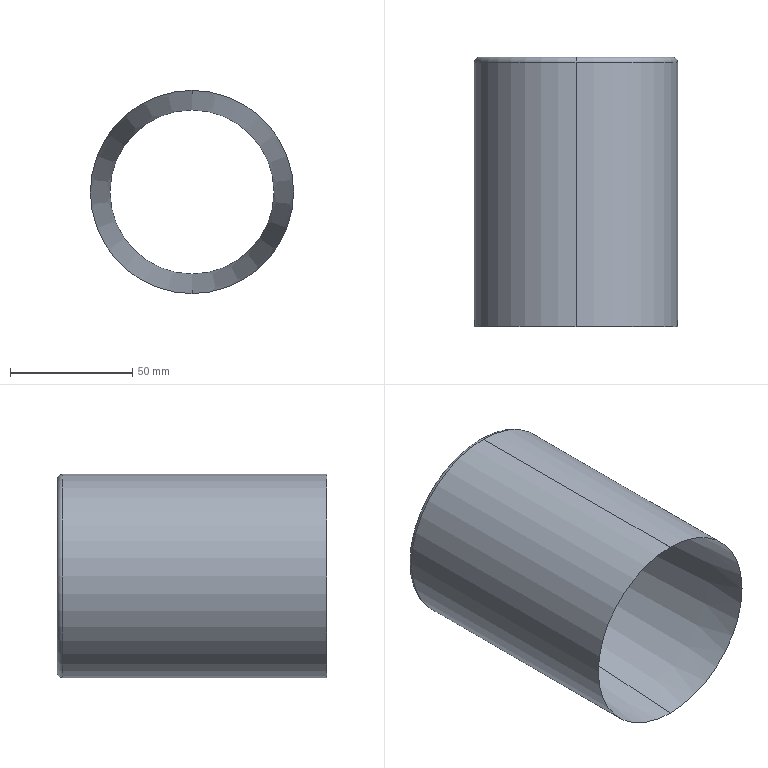Part | SolidWorks | features RevolutionThin 1 | 1 solid | 22 faces | box 83 x 110 x 83 mm | volume 48850 mm3 | cylinder 8 | torus 8 | cone 4 | plane 2 | commonest cylinder face diameters 67 x2 69 x2 81 x2 83 x2
STEP:
#1=CARTESIAN_POINT('',(0.,108.,33.5));
#2=VERTEX_POINT('',#1);
#3=CARTESIAN_POINT('',(0.,108.,-33.5));
#4=VERTEX_POINT('',#3);
#5=CARTESIAN_POINT('',(0.,108.,0.));
#6=DIRECTION('',(0.,-1.,0.));
#7=DIRECTION('',(0.,0.,-1.));
#8=AXIS2_PLACEMENT_3D('',#5,#6,#7);
#9=CIRCLE('',#8,33.5);
#10=EDGE_CURVE('',#2,#4,#9,.T.);
#11=ORIENTED_EDGE('',*,*,#10,.F.);
#12=CARTESIAN_POINT('',(0.,105.,33.5));
#13=VERTEX_POINT('',#12);
#14=CARTESIAN_POINT('',(0.,0.,33.5));
#15=DIRECTION('',(0.,-1.,0.));
#16=VECTOR('',#15,1000.);
#17=LINE('',#14,#16);
#18=EDGE_CURVE('',#2,#13,#17,.T.);
#19=ORIENTED_EDGE('',*,*,#18,.T.);
#20=CARTESIAN_POINT('',(0.,105.,-33.5));
#21=VERTEX_POINT('',#20);
#22=CARTESIAN_POINT('',(0.,105.,0.));
#23=DIRECTION('',(0.,-1.,0.));
#24=DIRECTION('',(0.,0.,-1.));
#25=AXIS2_PLACEMENT_3D('',#22,#23,#24);
#26=CIRCLE('',#25,33.5);
#27=EDGE_CURVE('',#13,#21,#26,.T.);
#28=ORIENTED_EDGE('',*,*,#27,.T.);
#29=CARTESIAN_POINT('',(0.,0.,-33.5));
#30=DIRECTION('',(0.,-1.,0.));
#31=VECTOR('',#30,1000.);
#32=LINE('',#29,#31);
#33=EDGE_CURVE('',#4,#21,#32,.T.);
#34=ORIENTED_EDGE('',*,*,#33,.F.);
#35=EDGE_LOOP('',(#11,#19,#28,#34));
#36=FACE_OUTER_BOUND('',#35,.T.);
#37=CARTESIAN_POINT('',(0.,0.,0.));
#38=DIRECTION('',(0.,-1.,0.));
#39=DIRECTION('',(0.,0.,-1.));
#40=AXIS2_PLACEMENT_3D('',#37,#38,#39);
#41=CYLINDRICAL_SURFACE('',#40,33.5);
#42=ADVANCED_FACE('',(#36),#41,.F.);
#43=CARTESIAN_POINT('',(0.,108.,0.));
#44=DIRECTION('',(0.,-1.,0.));
#45=DIRECTION('',(0.,0.,-1.));
#46=AXIS2_PLACEMENT_3D('',#43,#44,#45);
#47=CIRCLE('',#46,33.5);
#48=EDGE_CURVE('',#4,#2,#47,.T.);
#49=ORIENTED_EDGE('',*,*,#48,.T.);
#50=CARTESIAN_POINT('',(0.,110.,35.5));
#51=VERTEX_POINT('',#50);
#52=CARTESIAN_POINT('',(0.,108.,35.5));
#53=DIRECTION('',(1.,0.,0.));
#54=DIRECTION('',(0.,0.,-1.));
#55=AXIS2_PLACEMENT_3D('',#52,#53,#54);
#56=CIRCLE('',#55,2.);
#57=EDGE_CURVE('',#2,#51,#56,.T.);
#58=ORIENTED_EDGE('',*,*,#57,.T.);
#59=CARTESIAN_POINT('',(0.,110.,-35.5));
#60=VERTEX_POINT('',#59);
#61=CARTESIAN_POINT('',(0.,110.,0.));
#62=DIRECTION('',(0.,-1.,0.));
#63=DIRECTION('',(0.,0.,-1.));
#64=AXIS2_PLACEMENT_3D('',#61,#62,#63);
#65=CIRCLE('',#64,35.5);
#66=EDGE_CURVE('',#60,#51,#65,.T.);
#67=ORIENTED_EDGE('',*,*,#66,.F.);
#68=CARTESIAN_POINT('',(0.,108.,-35.5));
#69=DIRECTION('',(-1.,0.,0.));
#70=DIRECTION('',(0.,0.,1.));
#71=AXIS2_PLACEMENT_3D('',#68,#69,#70);
#72=CIRCLE('',#71,2.);
#73=EDGE_CURVE('',#4,#60,#72,.T.);
#74=ORIENTED_EDGE('',*,*,#73,.F.);
#75=EDGE_LOOP('',(#49,#58,#67,#74));
#76=FACE_OUTER_BOUND('',#75,.T.);
#77=CARTESIAN_POINT('',(0.,108.,0.));
#78=DIRECTION('',(0.,-1.,0.));
#79=DIRECTION('',(0.,0.,-1.));
#80=AXIS2_PLACEMENT_3D('',#77,#78,#79);
#81=TOROIDAL_SURFACE('',#80,35.5,2.);
#82=ADVANCED_FACE('',(#76),#81,.T.);
#83=CARTESIAN_POINT('',(0.,110.,-39.5));
#84=VERTEX_POINT('',#83);
#85=CARTESIAN_POINT('',(0.,110.,39.5));
#86=VERTEX_POINT('',#85);
#87=CARTESIAN_POINT('',(0.,110.,0.));
#88=DIRECTION('',(0.,-1.,0.));
#89=DIRECTION('',(0.,0.,-1.));
#90=AXIS2_PLACEMENT_3D('',#87,#88,#89);
#91=CIRCLE('',#90,39.5);
#92=EDGE_CURVE('',#84,#86,#91,.T.);
#93=ORIENTED_EDGE('',*,*,#92,.T.);
#94=CARTESIAN_POINT('',(0.,108.,41.5));
#95=VERTEX_POINT('',#94);
#96=CARTESIAN_POINT('',(0.,108.,39.5));
#97=DIRECTION('',(1.,0.,0.));
#98=DIRECTION('',(0.,0.,-1.));
#99=AXIS2_PLACEMENT_3D('',#96,#97,#98);
#100=CIRCLE('',#99,2.);
#101=EDGE_CURVE('',#86,#95,#100,.T.);
#102=ORIENTED_EDGE('',*,*,#101,.T.);
#103=CARTESIAN_POINT('',(0.,108.,-41.5));
#104=VERTEX_POINT('',#103);
#105=CARTESIAN_POINT('',(0.,108.,0.));
#106=DIRECTION('',(0.,-1.,0.));
#107=DIRECTION('',(0.,0.,-1.));
#108=AXIS2_PLACEMENT_3D('',#105,#106,#107);
#109=CIRCLE('',#108,41.5);
#110=EDGE_CURVE('',#104,#95,#109,.T.);
#111=ORIENTED_EDGE('',*,*,#110,.F.);
#112=CARTESIAN_POINT('',(0.,108.,-39.5));
#113=DIRECTION('',(-1.,0.,0.));
#114=DIRECTION('',(0.,0.,1.));
#115=AXIS2_PLACEMENT_3D('',#112,#113,#114);
#116=CIRCLE('',#115,2.);
#117=EDGE_CURVE('',#84,#104,#116,.T.);
#118=ORIENTED_EDGE('',*,*,#117,.F.);
#119=EDGE_LOOP('',(#93,#102,#111,#118));
#120=FACE_OUTER_BOUND('',#119,.T.);
#121=CARTESIAN_POINT('',(0.,108.,0.));
#122=DIRECTION('',(0.,-1.,0.));
#123=DIRECTION('',(0.,0.,-1.));
#124=AXIS2_PLACEMENT_3D('',#121,#122,#123);
#125=TOROIDAL_SURFACE('',#124,39.5,2.);
#126=ADVANCED_FACE('',(#120),#125,.T.);
#127=ORIENTED_EDGE('',*,*,#110,.T.);
#128=CARTESIAN_POINT('',(0.,0.,41.5));
#129=VERTEX_POINT('',#128);
#130=CARTESIAN_POINT('',(0.,0.,41.5));
#131=DIRECTION('',(0.,-1.,0.));
#132=VECTOR('',#131,1000.);
#133=LINE('',#130,#132);
#134=EDGE_CURVE('',#95,#129,#133,.T.);
#135=ORIENTED_EDGE('',*,*,#134,.T.);
#136=CARTESIAN_POINT('',(0.,0.,-41.5));
#137=VERTEX_POINT('',#136);
#138=CARTESIAN_POINT('',(0.,0.,0.));
#139=DIRECTION('',(0.,-1.,0.));
#140=DIRECTION('',(0.,0.,-1.));
#141=AXIS2_PLACEMENT_3D('',#138,#139,#140);
#142=CIRCLE('',#141,41.5);
#143=EDGE_CURVE('',#137,#129,#142,.T.);
#144=ORIENTED_EDGE('',*,*,#143,.F.);
#145=CARTESIAN_POINT('',(0.,0.,-41.5));
#146=DIRECTION('',(0.,-1.,0.));
#147=VECTOR('',#146,1000.);
#148=LINE('',#145,#147);
#149=EDGE_CURVE('',#104,#137,#148,.T.);
#150=ORIENTED_EDGE('',*,*,#149,.F.);
#151=EDGE_LOOP('',(#127,#135,#144,#150));
#152=FACE_OUTER_BOUND('',#151,.T.);
#153=CARTESIAN_POINT('',(0.,0.,0.));
#154=DIRECTION('',(0.,-1.,0.));
#155=DIRECTION('',(0.,0.,-1.));
#156=AXIS2_PLACEMENT_3D('',#153,#154,#155);
#157=CYLINDRICAL_SURFACE('',#156,41.5);
#158=ADVANCED_FACE('',(#152),#157,.T.);
#159=ORIENTED_EDGE('',*,*,#27,.F.);
#160=CARTESIAN_POINT('',(0.,105.,33.5));
#161=DIRECTION('',(0.,-0.9971,0.07597));
#162=VECTOR('',#161,1000.);
#163=LINE('',#160,#162);
#164=EDGE_CURVE('',#13,#129,#163,.T.);
#165=ORIENTED_EDGE('',*,*,#164,.T.);
#166=CARTESIAN_POINT('',(0.,0.,0.));
#167=DIRECTION('',(0.,-1.,0.));
#168=DIRECTION('',(0.,0.,-1.));
#169=AXIS2_PLACEMENT_3D('',#166,#167,#168);
#170=CIRCLE('',#169,41.5);
#171=EDGE_CURVE('',#129,#137,#170,.T.);
#172=ORIENTED_EDGE('',*,*,#171,.T.);
#173=CARTESIAN_POINT('',(0.,105.,-33.5));
#174=DIRECTION('',(0.,-0.9971,-0.07597));
#175=VECTOR('',#174,1000.);
#176=LINE('',#173,#175);
#177=EDGE_CURVE('',#21,#137,#176,.T.);
#178=ORIENTED_EDGE('',*,*,#177,.F.);
#179=EDGE_LOOP('',(#159,#165,#172,#178));
#180=FACE_OUTER_BOUND('',#179,.T.);
#181=CARTESIAN_POINT('',(0.,105.,0.));
#182=DIRECTION('',(0.,-1.,0.));
#183=DIRECTION('',(0.,0.,-1.));
#184=AXIS2_PLACEMENT_3D('',#181,#182,#183);
#185=CONICAL_SURFACE('',#184,33.5,0.07604);
#186=ADVANCED_FACE('',(#180),#185,.F.);
#187=ORIENTED_EDGE('',*,*,#164,.F.);
#188=CARTESIAN_POINT('',(0.,105.,0.));
#189=DIRECTION('',(0.,-1.,0.));
#190=DIRECTION('',(0.,0.,-1.));
#191=AXIS2_PLACEMENT_3D('',#188,#189,#190);
#192=CIRCLE('',#191,33.5);
#193=EDGE_CURVE('',#21,#13,#192,.T.);
#194=ORIENTED_EDGE('',*,*,#193,.F.);
#195=ORIENTED_EDGE('',*,*,#177,.T.);
#196=ORIENTED_EDGE('',*,*,#143,.T.);
#197=EDGE_LOOP('',(#187,#194,#195,#196));
#198=FACE_OUTER_BOUND('',#197,.T.);
#199=CARTESIAN_POINT('',(0.,105.,0.));
#200=DIRECTION('',(0.,-1.,0.));
#201=DIRECTION('',(0.,0.,-1.));
#202=AXIS2_PLACEMENT_3D('',#199,#200,#201);
#203=CONICAL_SURFACE('',#202,33.5,0.07604);
#204=ADVANCED_FACE('',(#198),#203,.F.);
#205=ORIENTED_EDGE('',*,*,#134,.F.);
#206=CARTESIAN_POINT('',(0.,108.,0.));
#207=DIRECTION('',(0.,-1.,0.));
#208=DIRECTION('',(0.,0.,-1.));
#209=AXIS2_PLACEMENT_3D('',#206,#207,#208);
#210=CIRCLE('',#209,41.5);
#211=EDGE_CURVE('',#95,#104,#210,.T.);
#212=ORIENTED_EDGE('',*,*,#211,.T.);
#213=ORIENTED_EDGE('',*,*,#149,.T.);
#214=ORIENTED_EDGE('',*,*,#171,.F.);
#215=EDGE_LOOP('',(#205,#212,#213,#214));
#216=FACE_OUTER_BOUND('',#215,.T.);
#217=CARTESIAN_POINT('',(0.,0.,0.));
#218=DIRECTION('',(0.,-1.,0.));
#219=DIRECTION('',(0.,0.,-1.));
#220=AXIS2_PLACEMENT_3D('',#217,#218,#219);
#221=CYLINDRICAL_SURFACE('',#220,41.5);
#222=ADVANCED_FACE('',(#216),#221,.T.);
#223=ORIENTED_EDGE('',*,*,#101,.F.);
#224=CARTESIAN_POINT('',(0.,110.,0.));
#225=DIRECTION('',(0.,-1.,0.));
#226=DIRECTION('',(0.,0.,-1.));
#227=AXIS2_PLACEMENT_3D('',#224,#225,#226);
#228=CIRCLE('',#227,39.5);
#229=EDGE_CURVE('',#86,#84,#228,.T.);
#230=ORIENTED_EDGE('',*,*,#229,.T.);
#231=ORIENTED_EDGE('',*,*,#117,.T.);
#232=ORIENTED_EDGE('',*,*,#211,.F.);
#233=EDGE_LOOP('',(#223,#230,#231,#232));
#234=FACE_OUTER_BOUND('',#233,.T.);
#235=CARTESIAN_POINT('',(0.,108.,0.));
#236=DIRECTION('',(0.,-1.,0.));
#237=DIRECTION('',(0.,0.,-1.));
#238=AXIS2_PLACEMENT_3D('',#235,#236,#237);
#239=TOROIDAL_SURFACE('',#238,39.5,2.);
#240=ADVANCED_FACE('',(#234),#239,.T.);
#241=ORIENTED_EDGE('',*,*,#66,.T.);
#242=CARTESIAN_POINT('',(0.,110.,0.));
#243=DIRECTION('',(0.,-1.,0.));
#244=DIRECTION('',(0.,0.,-1.));
#245=AXIS2_PLACEMENT_3D('',#242,#243,#244);
#246=CIRCLE('',#245,35.5);
#247=EDGE_CURVE('',#51,#60,#246,.T.);
#248=ORIENTED_EDGE('',*,*,#247,.T.);
#249=EDGE_LOOP('',(#241,#248));
#250=FACE_BOUND('',#249,.T.);
#251=ORIENTED_EDGE('',*,*,#92,.F.);
#252=ORIENTED_EDGE('',*,*,#229,.F.);
#253=EDGE_LOOP('',(#251,#252));
#254=FACE_OUTER_BOUND('',#253,.T.);
#255=CARTESIAN_POINT('',(39.5,110.,0.));
#256=DIRECTION('',(0.,1.,0.));
#257=DIRECTION('',(0.,0.,1.));
#258=AXIS2_PLACEMENT_3D('',#255,#256,#257);
#259=PLANE('',#258);
#260=ADVANCED_FACE('',(#250,#254),#259,.T.);
#261=ORIENTED_EDGE('',*,*,#57,.F.);
#262=ORIENTED_EDGE('',*,*,#10,.T.);
#263=ORIENTED_EDGE('',*,*,#73,.T.);
#264=ORIENTED_EDGE('',*,*,#247,.F.);
#265=EDGE_LOOP('',(#261,#262,#263,#264));
#266=FACE_OUTER_BOUND('',#265,.T.);
#267=CARTESIAN_POINT('',(0.,108.,0.));
#268=DIRECTION('',(0.,-1.,0.));
#269=DIRECTION('',(0.,0.,-1.));
#270=AXIS2_PLACEMENT_3D('',#267,#268,#269);
#271=TOROIDAL_SURFACE('',#270,35.5,2.);
#272=ADVANCED_FACE('',(#266),#271,.T.);
#273=ORIENTED_EDGE('',*,*,#18,.F.);
#274=ORIENTED_EDGE('',*,*,#48,.F.);
#275=ORIENTED_EDGE('',*,*,#33,.T.);
#276=ORIENTED_EDGE('',*,*,#193,.T.);
#277=EDGE_LOOP('',(#273,#274,#275,#276));
#278=FACE_OUTER_BOUND('',#277,.T.);
#279=CARTESIAN_POINT('',(0.,0.,0.));
#280=DIRECTION('',(0.,-1.,0.));
#281=DIRECTION('',(0.,0.,-1.));
#282=AXIS2_PLACEMENT_3D('',#279,#280,#281);
#283=CYLINDRICAL_SURFACE('',#282,33.5);
#284=ADVANCED_FACE('',(#278),#283,.F.);
#285=CLOSED_SHELL('',(#42,#82,#126,#158,#186,#204,#222,#240,#260,#272,#284));
#286=CARTESIAN_POINT('',(0.,108.,-34.5));
#287=VERTEX_POINT('',#286);
#288=CARTESIAN_POINT('',(0.,108.,34.5));
#289=VERTEX_POINT('',#288);
#290=CARTESIAN_POINT('',(0.,108.,0.));
#291=DIRECTION('',(0.,-1.,0.));
#292=DIRECTION('',(0.,0.,-1.));
#293=AXIS2_PLACEMENT_3D('',#290,#291,#292);
#294=CIRCLE('',#293,34.5);
#295=EDGE_CURVE('',#287,#289,#294,.T.);
#296=ORIENTED_EDGE('',*,*,#295,.T.);
#297=CARTESIAN_POINT('',(0.,105.038,34.5));
#298=VERTEX_POINT('',#297);
#299=CARTESIAN_POINT('',(0.,0.,34.5));
#300=DIRECTION('',(0.,-1.,0.));
#301=VECTOR('',#300,1000.);
#302=LINE('',#299,#301);
#303=EDGE_CURVE('',#289,#298,#302,.T.);
#304=ORIENTED_EDGE('',*,*,#303,.T.);
#305=CARTESIAN_POINT('',(0.,105.038,-34.5));
#306=VERTEX_POINT('',#305);
#307=CARTESIAN_POINT('',(0.,105.038,0.));
#308=DIRECTION('',(0.,-1.,0.));
#309=DIRECTION('',(0.,0.,-1.));
#310=AXIS2_PLACEMENT_3D('',#307,#308,#309);
#311=CIRCLE('',#310,34.5);
#312=EDGE_CURVE('',#306,#298,#311,.T.);
#313=ORIENTED_EDGE('',*,*,#312,.F.);
#314=CARTESIAN_POINT('',(0.,0.,-34.5));
#315=DIRECTION('',(0.,-1.,0.));
#316=VECTOR('',#315,1000.);
#317=LINE('',#314,#316);
#318=EDGE_CURVE('',#287,#306,#317,.T.);
#319=ORIENTED_EDGE('',*,*,#318,.F.);
#320=EDGE_LOOP('',(#296,#304,#313,#319));
#321=FACE_OUTER_BOUND('',#320,.T.);
#322=CARTESIAN_POINT('',(0.,0.,0.));
#323=DIRECTION('',(0.,-1.,0.));
#324=DIRECTION('',(0.,0.,-1.));
#325=AXIS2_PLACEMENT_3D('',#322,#323,#324);
#326=CYLINDRICAL_SURFACE('',#325,34.5);
#327=ADVANCED_FACE('',(#321),#326,.T.);
#328=CARTESIAN_POINT('',(0.,108.,0.));
#329=DIRECTION('',(0.,-1.,0.));
#330=DIRECTION('',(0.,0.,-1.));
#331=AXIS2_PLACEMENT_3D('',#328,#329,#330);
#332=CIRCLE('',#331,34.5);
#333=EDGE_CURVE('',#289,#287,#332,.T.);
#334=ORIENTED_EDGE('',*,*,#333,.F.);
#335=CARTESIAN_POINT('',(0.,109.,35.5));
#336=VERTEX_POINT('',#335);
#337=CARTESIAN_POINT('',(0.,108.,35.5));
#338=DIRECTION('',(1.,0.,0.));
#339=DIRECTION('',(0.,0.,-1.));
#340=AXIS2_PLACEMENT_3D('',#337,#338,#339);
#341=CIRCLE('',#340,1.);
#342=EDGE_CURVE('',#289,#336,#341,.T.);
#343=ORIENTED_EDGE('',*,*,#342,.T.);
#344=CARTESIAN_POINT('',(0.,109.,-35.5));
#345=VERTEX_POINT('',#344);
#346=CARTESIAN_POINT('',(0.,109.,0.));
#347=DIRECTION('',(0.,-1.,0.));
#348=DIRECTION('',(0.,0.,-1.));
#349=AXIS2_PLACEMENT_3D('',#346,#347,#348);
#350=CIRCLE('',#349,35.5);
#351=EDGE_CURVE('',#336,#345,#350,.T.);
#352=ORIENTED_EDGE('',*,*,#351,.T.);
#353=CARTESIAN_POINT('',(0.,108.,-35.5));
#354=DIRECTION('',(-1.,0.,0.));
#355=DIRECTION('',(0.,0.,1.));
#356=AXIS2_PLACEMENT_3D('',#353,#354,#355);
#357=CIRCLE('',#356,1.);
#358=EDGE_CURVE('',#287,#345,#357,.T.);
#359=ORIENTED_EDGE('',*,*,#358,.F.);
#360=EDGE_LOOP('',(#334,#343,#352,#359));
#361=FACE_OUTER_BOUND('',#360,.T.);
#362=CARTESIAN_POINT('',(0.,108.,0.));
#363=DIRECTION('',(0.,-1.,0.));
#364=DIRECTION('',(0.,0.,-1.));
#365=AXIS2_PLACEMENT_3D('',#362,#363,#364);
#366=TOROIDAL_SURFACE('',#365,35.5,1.);
#367=ADVANCED_FACE('',(#361),#366,.F.);
#368=CARTESIAN_POINT('',(0.,109.,39.5));
#369=VERTEX_POINT('',#368);
#370=CARTESIAN_POINT('',(0.,109.,-39.5));
#371=VERTEX_POINT('',#370);
#372=CARTESIAN_POINT('',(0.,109.,0.));
#373=DIRECTION('',(0.,-1.,0.));
#374=DIRECTION('',(0.,0.,-1.));
#375=AXIS2_PLACEMENT_3D('',#372,#373,#374);
#376=CIRCLE('',#375,39.5);
#377=EDGE_CURVE('',#369,#371,#376,.T.);
#378=ORIENTED_EDGE('',*,*,#377,.F.);
#379=CARTESIAN_POINT('',(0.,108.,40.5));
#380=VERTEX_POINT('',#379);
#381=CARTESIAN_POINT('',(0.,108.,39.5));
#382=DIRECTION('',(1.,0.,0.));
#383=DIRECTION('',(0.,0.,-1.));
#384=AXIS2_PLACEMENT_3D('',#381,#382,#383);
#385=CIRCLE('',#384,1.);
#386=EDGE_CURVE('',#369,#380,#385,.T.);
#387=ORIENTED_EDGE('',*,*,#386,.T.);
#388=CARTESIAN_POINT('',(0.,108.,-40.5));
#389=VERTEX_POINT('',#388);
#390=CARTESIAN_POINT('',(0.,108.,0.));
#391=DIRECTION('',(0.,-1.,0.));
#392=DIRECTION('',(0.,0.,-1.));
#393=AXIS2_PLACEMENT_3D('',#390,#391,#392);
#394=CIRCLE('',#393,40.5);
#395=EDGE_CURVE('',#380,#389,#394,.T.);
#396=ORIENTED_EDGE('',*,*,#395,.T.);
#397=CARTESIAN_POINT('',(0.,108.,-39.5));
#398=DIRECTION('',(-1.,0.,0.));
#399=DIRECTION('',(0.,0.,1.));
#400=AXIS2_PLACEMENT_3D('',#397,#398,#399);
#401=CIRCLE('',#400,1.);
#402=EDGE_CURVE('',#371,#389,#401,.T.);
#403=ORIENTED_EDGE('',*,*,#402,.F.);
#404=EDGE_LOOP('',(#378,#387,#396,#403));
#405=FACE_OUTER_BOUND('',#404,.T.);
#406=CARTESIAN_POINT('',(0.,108.,0.));
#407=DIRECTION('',(0.,-1.,0.));
#408=DIRECTION('',(0.,0.,-1.));
#409=AXIS2_PLACEMENT_3D('',#406,#407,#408);
#410=TOROIDAL_SURFACE('',#409,39.5,1.);
#411=ADVANCED_FACE('',(#405),#410,.F.);
#412=ORIENTED_EDGE('',*,*,#395,.F.);
#413=CARTESIAN_POINT('',(0.,26.288,40.5));
#414=VERTEX_POINT('',#413);
#415=CARTESIAN_POINT('',(0.,0.,40.5));
#416=DIRECTION('',(0.,-1.,0.));
#417=VECTOR('',#416,1000.);
#418=LINE('',#415,#417);
#419=EDGE_CURVE('',#380,#414,#418,.T.);
#420=ORIENTED_EDGE('',*,*,#419,.T.);
#421=CARTESIAN_POINT('',(0.,26.288,-40.5));
#422=VERTEX_POINT('',#421);
#423=CARTESIAN_POINT('',(0.,26.288,0.));
#424=DIRECTION('',(0.,-1.,0.));
#425=DIRECTION('',(0.,0.,-1.));
#426=AXIS2_PLACEMENT_3D('',#423,#424,#425);
#427=CIRCLE('',#426,40.5);
#428=EDGE_CURVE('',#414,#422,#427,.T.);
#429=ORIENTED_EDGE('',*,*,#428,.T.);
#430=CARTESIAN_POINT('',(0.,0.,-40.5));
#431=DIRECTION('',(0.,-1.,0.));
#432=VECTOR('',#431,1000.);
#433=LINE('',#430,#432);
#434=EDGE_CURVE('',#389,#422,#433,.T.);
#435=ORIENTED_EDGE('',*,*,#434,.F.);
#436=EDGE_LOOP('',(#412,#420,#429,#435));
#437=FACE_OUTER_BOUND('',#436,.T.);
#438=CARTESIAN_POINT('',(0.,0.,0.));
#439=DIRECTION('',(0.,-1.,0.));
#440=DIRECTION('',(0.,0.,-1.));
#441=AXIS2_PLACEMENT_3D('',#438,#439,#440);
#442=CYLINDRICAL_SURFACE('',#441,40.5);
#443=ADVANCED_FACE('',(#437),#442,.F.);
#444=ORIENTED_EDGE('',*,*,#312,.T.);
#445=CARTESIAN_POINT('',(0.,105.038,34.5));
#446=DIRECTION('',(0.,-0.9971,0.07597));
#447=VECTOR('',#446,1000.);
#448=LINE('',#445,#447);
#449=EDGE_CURVE('',#298,#414,#448,.T.);
#450=ORIENTED_EDGE('',*,*,#449,.T.);
#451=CARTESIAN_POINT('',(0.,26.288,0.));
#452=DIRECTION('',(0.,-1.,0.));
#453=DIRECTION('',(0.,0.,-1.));
#454=AXIS2_PLACEMENT_3D('',#451,#452,#453);
#455=CIRCLE('',#454,40.5);
#456=EDGE_CURVE('',#422,#414,#455,.T.);
#457=ORIENTED_EDGE('',*,*,#456,.F.);
#458=CARTESIAN_POINT('',(0.,105.038,-34.5));
#459=DIRECTION('',(0.,-0.9971,-0.07597));
#460=VECTOR('',#459,1000.);
#461=LINE('',#458,#460);
#462=EDGE_CURVE('',#306,#422,#461,.T.);
#463=ORIENTED_EDGE('',*,*,#462,.F.);
#464=EDGE_LOOP('',(#444,#450,#457,#463));
#465=FACE_OUTER_BOUND('',#464,.T.);
#466=CARTESIAN_POINT('',(0.,105.038,0.));
#467=DIRECTION('',(0.,-1.,0.));
#468=DIRECTION('',(0.,0.,-1.));
#469=AXIS2_PLACEMENT_3D('',#466,#467,#468);
#470=CONICAL_SURFACE('',#469,34.5,0.07604);
#471=ADVANCED_FACE('',(#465),#470,.T.);
#472=ORIENTED_EDGE('',*,*,#449,.F.);
#473=CARTESIAN_POINT('',(0.,105.038,0.));
#474=DIRECTION('',(0.,-1.,0.));
#475=DIRECTION('',(0.,0.,-1.));
#476=AXIS2_PLACEMENT_3D('',#473,#474,#475);
#477=CIRCLE('',#476,34.5);
#478=EDGE_CURVE('',#298,#306,#477,.T.);
#479=ORIENTED_EDGE('',*,*,#478,.T.);
#480=ORIENTED_EDGE('',*,*,#462,.T.);
#481=ORIENTED_EDGE('',*,*,#428,.F.);
#482=EDGE_LOOP('',(#472,#479,#480,#481));
#483=FACE_OUTER_BOUND('',#482,.T.);
#484=CARTESIAN_POINT('',(0.,105.038,0.));
#485=DIRECTION('',(0.,-1.,0.));
#486=DIRECTION('',(0.,0.,-1.));
#487=AXIS2_PLACEMENT_3D('',#484,#485,#486);
#488=CONICAL_SURFACE('',#487,34.5,0.07604);
#489=ADVANCED_FACE('',(#483),#488,.T.);
#490=ORIENTED_EDGE('',*,*,#419,.F.);
#491=CARTESIAN_POINT('',(0.,108.,0.));
#492=DIRECTION('',(0.,-1.,0.));
#493=DIRECTION('',(0.,0.,-1.));
#494=AXIS2_PLACEMENT_3D('',#491,#492,#493);
#495=CIRCLE('',#494,40.5);
#496=EDGE_CURVE('',#389,#380,#495,.T.);
#497=ORIENTED_EDGE('',*,*,#496,.F.);
#498=ORIENTED_EDGE('',*,*,#434,.T.);
#499=ORIENTED_EDGE('',*,*,#456,.T.);
#500=EDGE_LOOP('',(#490,#497,#498,#499));
#501=FACE_OUTER_BOUND('',#500,.T.);
#502=CARTESIAN_POINT('',(0.,0.,0.));
#503=DIRECTION('',(0.,-1.,0.));
#504=DIRECTION('',(0.,0.,-1.));
#505=AXIS2_PLACEMENT_3D('',#502,#503,#504);
#506=CYLINDRICAL_SURFACE('',#505,40.5);
#507=ADVANCED_FACE('',(#501),#506,.F.);
#508=ORIENTED_EDGE('',*,*,#386,.F.);
#509=CARTESIAN_POINT('',(0.,109.,0.));
#510=DIRECTION('',(0.,-1.,0.));
#511=DIRECTION('',(0.,0.,-1.));
#512=AXIS2_PLACEMENT_3D('',#509,#510,#511);
#513=CIRCLE('',#512,39.5);
#514=EDGE_CURVE('',#371,#369,#513,.T.);
#515=ORIENTED_EDGE('',*,*,#514,.F.);
#516=ORIENTED_EDGE('',*,*,#402,.T.);
#517=ORIENTED_EDGE('',*,*,#496,.T.);
#518=EDGE_LOOP('',(#508,#515,#516,#517));
#519=FACE_OUTER_BOUND('',#518,.T.);
#520=CARTESIAN_POINT('',(0.,108.,0.));
#521=DIRECTION('',(0.,-1.,0.));
#522=DIRECTION('',(0.,0.,-1.));
#523=AXIS2_PLACEMENT_3D('',#520,#521,#522);
#524=TOROIDAL_SURFACE('',#523,39.5,1.);
#525=ADVANCED_FACE('',(#519),#524,.F.);
#526=CARTESIAN_POINT('',(0.,109.,0.));
#527=DIRECTION('',(0.,-1.,0.));
#528=DIRECTION('',(0.,0.,-1.));
#529=AXIS2_PLACEMENT_3D('',#526,#527,#528);
#530=CIRCLE('',#529,35.5);
#531=EDGE_CURVE('',#345,#336,#530,.T.);
#532=ORIENTED_EDGE('',*,*,#531,.F.);
#533=ORIENTED_EDGE('',*,*,#351,.F.);
#534=EDGE_LOOP('',(#532,#533));
#535=FACE_BOUND('',#534,.T.);
#536=ORIENTED_EDGE('',*,*,#514,.T.);
#537=ORIENTED_EDGE('',*,*,#377,.T.);
#538=EDGE_LOOP('',(#536,#537));
#539=FACE_OUTER_BOUND('',#538,.T.);
#540=CARTESIAN_POINT('',(39.5,109.,0.));
#541=DIRECTION('',(0.,1.,0.));
#542=DIRECTION('',(0.,0.,1.));
#543=AXIS2_PLACEMENT_3D('',#540,#541,#542);
#544=PLANE('',#543);
#545=ADVANCED_FACE('',(#535,#539),#544,.F.);
#546=ORIENTED_EDGE('',*,*,#342,.F.);
#547=ORIENTED_EDGE('',*,*,#295,.F.);
#548=ORIENTED_EDGE('',*,*,#358,.T.);
#549=ORIENTED_EDGE('',*,*,#531,.T.);
#550=EDGE_LOOP('',(#546,#547,#548,#549));
#551=FACE_OUTER_BOUND('',#550,.T.);
#552=CARTESIAN_POINT('',(0.,108.,0.));
#553=DIRECTION('',(0.,-1.,0.));
#554=DIRECTION('',(0.,0.,-1.));
#555=AXIS2_PLACEMENT_3D('',#552,#553,#554);
#556=TOROIDAL_SURFACE('',#555,35.5,1.);
#557=ADVANCED_FACE('',(#551),#556,.F.);
#558=ORIENTED_EDGE('',*,*,#303,.F.);
#559=ORIENTED_EDGE('',*,*,#333,.T.);
#560=ORIENTED_EDGE('',*,*,#318,.T.);
#561=ORIENTED_EDGE('',*,*,#478,.F.);
#562=EDGE_LOOP('',(#558,#559,#560,#561));
#563=FACE_OUTER_BOUND('',#562,.T.);
#564=CARTESIAN_POINT('',(0.,0.,0.));
#565=DIRECTION('',(0.,-1.,0.));
#566=DIRECTION('',(0.,0.,-1.));
#567=AXIS2_PLACEMENT_3D('',#564,#565,#566);
#568=CYLINDRICAL_SURFACE('',#567,34.5);
#569=ADVANCED_FACE('',(#563),#568,.T.);
#570=CLOSED_SHELL('',(#327,#367,#411,#443,#471,#489,#507,#525,#545,#557,#569));
#571=ORIENTED_CLOSED_SHELL('',*,#570,.F.);
#572=BREP_WITH_VOIDS('',#285,(#571));
#573=CARTESIAN_POINT('',(0.,0.,0.));
#574=DIRECTION('',(0.,0.,1.));
#575=DIRECTION('',(1.,0.,0.));
#576=AXIS2_PLACEMENT_3D('',#573,#574,#575);
#577=(LENGTH_UNIT()NAMED_UNIT(*)SI_UNIT(.MILLI.,.METRE.));
#578=UNCERTAINTY_MEASURE_WITH_UNIT(LENGTH_MEASURE(0.00001),#577,'','');
#579=(NAMED_UNIT(*)PLANE_ANGLE_UNIT()SI_UNIT($,.RADIAN.));
#580=(NAMED_UNIT(*)SI_UNIT($,.STERADIAN.)SOLID_ANGLE_UNIT());
#581=(GEOMETRIC_REPRESENTATION_CONTEXT(3)GLOBAL_UNCERTAINTY_ASSIGNED_CONTEXT((#578))GLOBAL_UNIT_ASSIGNED_CONTEXT((#577,#579,#580))REPRESENTATION_CONTEXT('',''));
#582=ADVANCED_BREP_SHAPE_REPRESENTATION('',(#572,#576),#581);